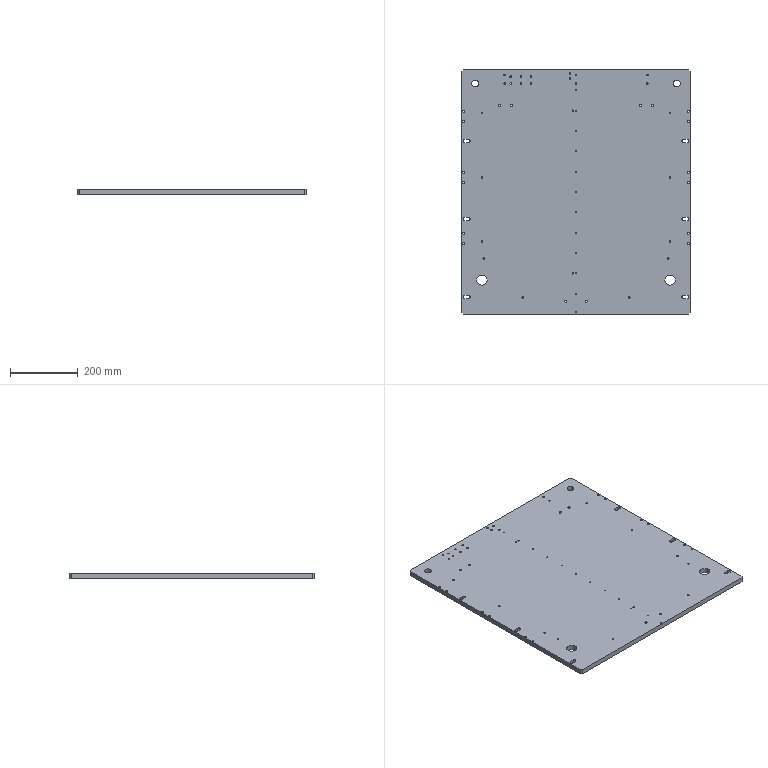Part | 1 solid | 94 faces | box 675 x 720 x 15 mm | volume 7226597 mm3 | cylinder 72 | plane 22 | commonest cylinder face diameters 5 x37 10 x12 3.3 x11 6.8 x6 4 x2 20 x2